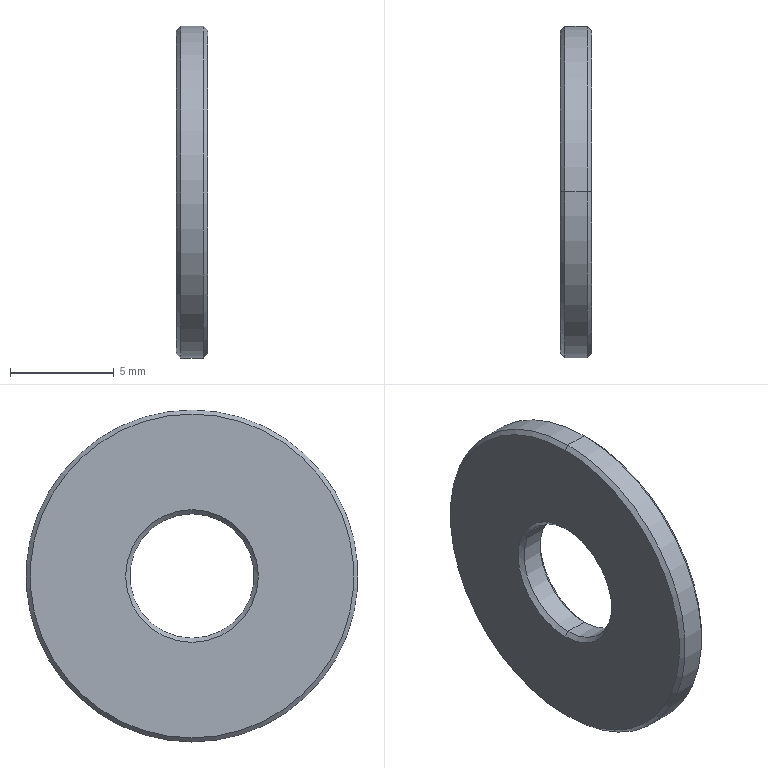Part | STEP file | WSSS16-6-1.5 | 1 solid | 14 faces | box 1.5 x 16 x 16 mm | volume 256.417 mm3 | cone 8 | cylinder 4 | plane 2 | commonest cylinder face diameters 6 x2 16 x2
STEP:
#1=CARTESIAN_POINT('',(0.,0.,0.));
#2=DIRECTION('',(0.,0.,1.));
#3=DIRECTION('',(1.,0.,0.));
#4=AXIS2_PLACEMENT_3D('',#1,#2,#3);
#5=CARTESIAN_POINT('',(1.5,0.,-7.8));
#6=VERTEX_POINT('',#5);
#7=CARTESIAN_POINT('',(1.5,0.,7.8));
#8=VERTEX_POINT('',#7);
#9=CARTESIAN_POINT('',(1.5,0.,0.));
#10=DIRECTION('',(1.,0.,0.));
#11=DIRECTION('',(0.,0.,1.));
#12=AXIS2_PLACEMENT_3D('',#9,#10,#11);
#13=CIRCLE('',#12,7.8);
#14=CARTESIAN_POINT('',(1.3,0.,0.));
#15=DIRECTION('',(-1.,0.,0.));
#16=DIRECTION('',(0.,0.,1.));
#17=AXIS2_PLACEMENT_3D('',#14,#15,#16);
#18=CONICAL_SURFACE('',#17,8.,0.7854);
#19=CARTESIAN_POINT('',(6.283,-0.2));
#20=DIRECTION('',(-1.,0.));
#21=VECTOR('',#20,1.);
#22=LINE('',#19,#21);
#23=(GEOMETRIC_REPRESENTATION_CONTEXT(2)PARAMETRIC_REPRESENTATION_CONTEXT()REPRESENTATION_CONTEXT('',''));
#24=DEFINITIONAL_REPRESENTATION('',(#22),#23);
#25=PCURVE('',#18,#24);
#26=CARTESIAN_POINT('',(1.5,3.,0.));
#27=DIRECTION('',(-1.,0.,0.));
#28=DIRECTION('',(0.,0.,1.));
#29=AXIS2_PLACEMENT_3D('',#26,#27,#28);
#30=PLANE('',#29);
#31=CARTESIAN_POINT('',(7.8,-3.));
#32=CARTESIAN_POINT('',(7.8,-16.51));
#33=CARTESIAN_POINT('',(-3.9,-9.755));
#34=CARTESIAN_POINT('',(-15.6,-3.));
#35=CARTESIAN_POINT('',(-3.9,3.755));
#36=CARTESIAN_POINT('',(7.8,10.51));
#37=CARTESIAN_POINT('',(7.8,-3.));
#38=(BOUNDED_CURVE()B_SPLINE_CURVE(2,(#31,#32,#33,#34,#35,#36,#37),.UNSPECIFIED.,.T.,.F.)B_SPLINE_CURVE_WITH_KNOTS((1,2,2,2,2,1),(-2.094,0.,2.094,4.189,6.283,8.378),.UNSPECIFIED.)CURVE()GEOMETRIC_REPRESENTATION_ITEM()RATIONAL_B_SPLINE_CURVE((1.,0.5,1.,0.5,1.,0.5,1.))REPRESENTATION_ITEM(''));
#39=(GEOMETRIC_REPRESENTATION_CONTEXT(2)PARAMETRIC_REPRESENTATION_CONTEXT()REPRESENTATION_CONTEXT('',''));
#40=DEFINITIONAL_REPRESENTATION('',(#38),#39);
#41=PCURVE('',#30,#40);
#42=SURFACE_CURVE('',#13,(#25,#41),.PCURVE_S1.);
#43=EDGE_CURVE('',#6,#8,#42,.T.);
#44=ORIENTED_EDGE('',*,*,#43,.F.);
#45=CARTESIAN_POINT('',(1.3,0.,-8.));
#46=VERTEX_POINT('',#45);
#47=CARTESIAN_POINT('',(1.3,0.,-8.));
#48=DIRECTION('',(-0.7071,0.,-0.7071));
#49=VECTOR('',#48,1.);
#50=LINE('',#47,#49);
#51=CARTESIAN_POINT('',(3.142,0.));
#52=DIRECTION('',(0.,1.));
#53=VECTOR('',#52,1.);
#54=LINE('',#51,#53);
#55=(GEOMETRIC_REPRESENTATION_CONTEXT(2)PARAMETRIC_REPRESENTATION_CONTEXT()REPRESENTATION_CONTEXT('',''));
#56=DEFINITIONAL_REPRESENTATION('',(#54),#55);
#57=PCURVE('',#18,#56);
#58=CARTESIAN_POINT('',(1.3,0.,0.));
#59=DIRECTION('',(-1.,0.,0.));
#60=DIRECTION('',(0.,0.,1.));
#61=AXIS2_PLACEMENT_3D('',#58,#59,#60);
#62=CONICAL_SURFACE('',#61,8.,0.7854);
#63=CARTESIAN_POINT('',(3.142,0.));
#64=DIRECTION('',(0.,1.));
#65=VECTOR('',#64,1.);
#66=LINE('',#63,#65);
#67=(GEOMETRIC_REPRESENTATION_CONTEXT(2)PARAMETRIC_REPRESENTATION_CONTEXT()REPRESENTATION_CONTEXT('',''));
#68=DEFINITIONAL_REPRESENTATION('',(#66),#67);
#69=PCURVE('',#62,#68);
#70=SURFACE_CURVE('',#50,(#57,#69),.PCURVE_S1.);
#71=EDGE_CURVE('',#6,#46,#70,.T.);
#72=ORIENTED_EDGE('',*,*,#71,.T.);
#73=CARTESIAN_POINT('',(1.3,0.,8.));
#74=VERTEX_POINT('',#73);
#75=CARTESIAN_POINT('',(1.3,0.,0.));
#76=DIRECTION('',(-1.,0.,0.));
#77=DIRECTION('',(0.,0.,1.));
#78=AXIS2_PLACEMENT_3D('',#75,#76,#77);
#79=CIRCLE('',#78,8.);
#80=CARTESIAN_POINT('',(0.,0.));
#81=DIRECTION('',(1.,0.));
#82=VECTOR('',#81,1.);
#83=LINE('',#80,#82);
#84=(GEOMETRIC_REPRESENTATION_CONTEXT(2)PARAMETRIC_REPRESENTATION_CONTEXT()REPRESENTATION_CONTEXT('',''));
#85=DEFINITIONAL_REPRESENTATION('',(#83),#84);
#86=PCURVE('',#18,#85);
#87=CARTESIAN_POINT('',(0.,0.,0.));
#88=DIRECTION('',(-1.,0.,0.));
#89=DIRECTION('',(0.,0.,1.));
#90=AXIS2_PLACEMENT_3D('',#87,#88,#89);
#91=CYLINDRICAL_SURFACE('',#90,8.);
#92=CARTESIAN_POINT('',(0.,-1.3));
#93=DIRECTION('',(1.,0.));
#94=VECTOR('',#93,1.);
#95=LINE('',#92,#94);
#96=(GEOMETRIC_REPRESENTATION_CONTEXT(2)PARAMETRIC_REPRESENTATION_CONTEXT()REPRESENTATION_CONTEXT('',''));
#97=DEFINITIONAL_REPRESENTATION('',(#95),#96);
#98=PCURVE('',#91,#97);
#99=SURFACE_CURVE('',#79,(#86,#98),.PCURVE_S1.);
#100=EDGE_CURVE('',#74,#46,#99,.T.);
#101=ORIENTED_EDGE('',*,*,#100,.F.);
#102=CARTESIAN_POINT('',(1.3,0.,8.));
#103=DIRECTION('',(-0.7071,0.,0.7071));
#104=VECTOR('',#103,1.);
#105=LINE('',#102,#104);
#106=CARTESIAN_POINT('',(0.,0.));
#107=DIRECTION('',(0.,1.));
#108=VECTOR('',#107,1.);
#109=LINE('',#106,#108);
#110=(GEOMETRIC_REPRESENTATION_CONTEXT(2)PARAMETRIC_REPRESENTATION_CONTEXT()REPRESENTATION_CONTEXT('',''));
#111=DEFINITIONAL_REPRESENTATION('',(#109),#110);
#112=PCURVE('',#18,#111);
#113=CARTESIAN_POINT('',(6.283,0.));
#114=DIRECTION('',(0.,1.));
#115=VECTOR('',#114,1.);
#116=LINE('',#113,#115);
#117=(GEOMETRIC_REPRESENTATION_CONTEXT(2)PARAMETRIC_REPRESENTATION_CONTEXT()REPRESENTATION_CONTEXT('',''));
#118=DEFINITIONAL_REPRESENTATION('',(#116),#117);
#119=PCURVE('',#62,#118);
#120=SURFACE_CURVE('',#105,(#112,#119),.PCURVE_S1.);
#121=EDGE_CURVE('',#8,#74,#120,.T.);
#122=ORIENTED_EDGE('',*,*,#121,.F.);
#123=EDGE_LOOP('',(#44,#72,#101,#122));
#124=FACE_BOUND('',#123,.T.);
#125=ADVANCED_FACE('',(#124),#18,.T.);
#126=CARTESIAN_POINT('',(1.3,0.,-3.));
#127=VERTEX_POINT('',#126);
#128=CARTESIAN_POINT('',(1.5,0.,-3.2));
#129=VERTEX_POINT('',#128);
#130=CARTESIAN_POINT('',(1.5,0.,-3.2));
#131=DIRECTION('',(0.7071,0.,-0.7071));
#132=VECTOR('',#131,1.);
#133=LINE('',#130,#132);
#134=CARTESIAN_POINT('',(1.5,0.,0.));
#135=DIRECTION('',(1.,0.,0.));
#136=DIRECTION('',(0.,0.,-1.));
#137=AXIS2_PLACEMENT_3D('',#134,#135,#136);
#138=CONICAL_SURFACE('',#137,3.2,0.7854);
#139=CARTESIAN_POINT('',(6.283,0.));
#140=DIRECTION('',(0.,1.));
#141=VECTOR('',#140,1.);
#142=LINE('',#139,#141);
#143=(GEOMETRIC_REPRESENTATION_CONTEXT(2)PARAMETRIC_REPRESENTATION_CONTEXT()REPRESENTATION_CONTEXT('',''));
#144=DEFINITIONAL_REPRESENTATION('',(#142),#143);
#145=PCURVE('',#138,#144);
#146=CARTESIAN_POINT('',(1.5,0.,0.));
#147=DIRECTION('',(1.,0.,0.));
#148=DIRECTION('',(0.,0.,-1.));
#149=AXIS2_PLACEMENT_3D('',#146,#147,#148);
#150=CONICAL_SURFACE('',#149,3.2,0.7854);
#151=CARTESIAN_POINT('',(0.,0.));
#152=DIRECTION('',(0.,1.));
#153=VECTOR('',#152,1.);
#154=LINE('',#151,#153);
#155=(GEOMETRIC_REPRESENTATION_CONTEXT(2)PARAMETRIC_REPRESENTATION_CONTEXT()REPRESENTATION_CONTEXT('',''));
#156=DEFINITIONAL_REPRESENTATION('',(#154),#155);
#157=PCURVE('',#150,#156);
#158=SURFACE_CURVE('',#133,(#145,#157),.PCURVE_S1.);
#159=EDGE_CURVE('',#127,#129,#158,.T.);
#160=ORIENTED_EDGE('',*,*,#159,.T.);
#161=CARTESIAN_POINT('',(1.5,0.,3.2));
#162=VERTEX_POINT('',#161);
#163=CARTESIAN_POINT('',(1.5,0.,0.));
#164=DIRECTION('',(-1.,0.,0.));
#165=DIRECTION('',(0.,0.,1.));
#166=AXIS2_PLACEMENT_3D('',#163,#164,#165);
#167=CIRCLE('',#166,3.2);
#168=CARTESIAN_POINT('',(9.425,0.));
#169=DIRECTION('',(-1.,0.));
#170=VECTOR('',#169,1.);
#171=LINE('',#168,#170);
#172=(GEOMETRIC_REPRESENTATION_CONTEXT(2)PARAMETRIC_REPRESENTATION_CONTEXT()REPRESENTATION_CONTEXT('',''));
#173=DEFINITIONAL_REPRESENTATION('',(#171),#172);
#174=PCURVE('',#138,#173);
#175=CARTESIAN_POINT('',(0.,-3.));
#176=DIRECTION('',(1.,0.));
#177=AXIS2_PLACEMENT_2D('',#175,#176);
#178=CIRCLE('',#177,3.2);
#179=(GEOMETRIC_REPRESENTATION_CONTEXT(2)PARAMETRIC_REPRESENTATION_CONTEXT()REPRESENTATION_CONTEXT('',''));
#180=DEFINITIONAL_REPRESENTATION('',(#178),#179);
#181=PCURVE('',#30,#180);
#182=SURFACE_CURVE('',#167,(#174,#181),.PCURVE_S1.);
#183=EDGE_CURVE('',#129,#162,#182,.T.);
#184=ORIENTED_EDGE('',*,*,#183,.T.);
#185=CARTESIAN_POINT('',(1.3,0.,3.));
#186=VERTEX_POINT('',#185);
#187=CARTESIAN_POINT('',(1.5,0.,3.2));
#188=DIRECTION('',(0.7071,0.,0.7071));
#189=VECTOR('',#188,1.);
#190=LINE('',#187,#189);
#191=CARTESIAN_POINT('',(3.142,0.));
#192=DIRECTION('',(0.,1.));
#193=VECTOR('',#192,1.);
#194=LINE('',#191,#193);
#195=(GEOMETRIC_REPRESENTATION_CONTEXT(2)PARAMETRIC_REPRESENTATION_CONTEXT()REPRESENTATION_CONTEXT('',''));
#196=DEFINITIONAL_REPRESENTATION('',(#194),#195);
#197=PCURVE('',#138,#196);
#198=CARTESIAN_POINT('',(3.142,0.));
#199=DIRECTION('',(0.,1.));
#200=VECTOR('',#199,1.);
#201=LINE('',#198,#200);
#202=(GEOMETRIC_REPRESENTATION_CONTEXT(2)PARAMETRIC_REPRESENTATION_CONTEXT()REPRESENTATION_CONTEXT('',''));
#203=DEFINITIONAL_REPRESENTATION('',(#201),#202);
#204=PCURVE('',#150,#203);
#205=SURFACE_CURVE('',#190,(#197,#204),.PCURVE_S1.);
#206=EDGE_CURVE('',#186,#162,#205,.T.);
#207=ORIENTED_EDGE('',*,*,#206,.F.);
#208=CARTESIAN_POINT('',(1.3,0.,0.));
#209=DIRECTION('',(1.,0.,0.));
#210=DIRECTION('',(0.,0.,1.));
#211=AXIS2_PLACEMENT_3D('',#208,#209,#210);
#212=CIRCLE('',#211,3.);
#213=CARTESIAN_POINT('',(3.142,-0.2));
#214=DIRECTION('',(1.,0.));
#215=VECTOR('',#214,1.);
#216=LINE('',#213,#215);
#217=(GEOMETRIC_REPRESENTATION_CONTEXT(2)PARAMETRIC_REPRESENTATION_CONTEXT()REPRESENTATION_CONTEXT('',''));
#218=DEFINITIONAL_REPRESENTATION('',(#216),#217);
#219=PCURVE('',#138,#218);
#220=CARTESIAN_POINT('',(0.,0.,0.));
#221=DIRECTION('',(-1.,0.,0.));
#222=DIRECTION('',(0.,0.,1.));
#223=AXIS2_PLACEMENT_3D('',#220,#221,#222);
#224=CYLINDRICAL_SURFACE('',#223,3.);
#225=CARTESIAN_POINT('',(6.283,-1.3));
#226=DIRECTION('',(-1.,0.));
#227=VECTOR('',#226,1.);
#228=LINE('',#225,#227);
#229=(GEOMETRIC_REPRESENTATION_CONTEXT(2)PARAMETRIC_REPRESENTATION_CONTEXT()REPRESENTATION_CONTEXT('',''));
#230=DEFINITIONAL_REPRESENTATION('',(#228),#229);
#231=PCURVE('',#224,#230);
#232=SURFACE_CURVE('',#212,(#219,#231),.PCURVE_S1.);
#233=EDGE_CURVE('',#186,#127,#232,.T.);
#234=ORIENTED_EDGE('',*,*,#233,.T.);
#235=EDGE_LOOP('',(#160,#184,#207,#234));
#236=FACE_BOUND('',#235,.F.);
#237=ADVANCED_FACE('',(#236),#138,.F.);
#238=CARTESIAN_POINT('',(0.,0.,7.8));
#239=VERTEX_POINT('',#238);
#240=CARTESIAN_POINT('',(0.,0.,-7.8));
#241=VERTEX_POINT('',#240);
#242=CARTESIAN_POINT('',(0.,0.,0.));
#243=DIRECTION('',(-1.,0.,0.));
#244=DIRECTION('',(0.,0.,-1.));
#245=AXIS2_PLACEMENT_3D('',#242,#243,#244);
#246=CIRCLE('',#245,7.8);
#247=CARTESIAN_POINT('',(0.,0.,0.));
#248=DIRECTION('',(1.,0.,0.));
#249=DIRECTION('',(0.,0.,-1.));
#250=AXIS2_PLACEMENT_3D('',#247,#248,#249);
#251=CONICAL_SURFACE('',#250,7.8,0.7854);
#252=CARTESIAN_POINT('',(6.283,0.));
#253=DIRECTION('',(-1.,0.));
#254=VECTOR('',#253,1.);
#255=LINE('',#252,#254);
#256=(GEOMETRIC_REPRESENTATION_CONTEXT(2)PARAMETRIC_REPRESENTATION_CONTEXT()REPRESENTATION_CONTEXT('',''));
#257=DEFINITIONAL_REPRESENTATION('',(#255),#256);
#258=PCURVE('',#251,#257);
#259=CARTESIAN_POINT('',(0.,3.,0.));
#260=DIRECTION('',(1.,0.,0.));
#261=DIRECTION('',(0.,0.,-1.));
#262=AXIS2_PLACEMENT_3D('',#259,#260,#261);
#263=PLANE('',#262);
#264=CARTESIAN_POINT('',(7.8,-3.));
#265=CARTESIAN_POINT('',(7.8,-16.51));
#266=CARTESIAN_POINT('',(-3.9,-9.755));
#267=CARTESIAN_POINT('',(-15.6,-3.));
#268=CARTESIAN_POINT('',(-3.9,3.755));
#269=CARTESIAN_POINT('',(7.8,10.51));
#270=CARTESIAN_POINT('',(7.8,-3.));
#271=(BOUNDED_CURVE()B_SPLINE_CURVE(2,(#264,#265,#266,#267,#268,#269,#270),.UNSPECIFIED.,.T.,.F.)B_SPLINE_CURVE_WITH_KNOTS((1,2,2,2,2,1),(-2.094,0.,2.094,4.189,6.283,8.378),.UNSPECIFIED.)CURVE()GEOMETRIC_REPRESENTATION_ITEM()RATIONAL_B_SPLINE_CURVE((1.,0.5,1.,0.5,1.,0.5,1.))REPRESENTATION_ITEM(''));
#272=(GEOMETRIC_REPRESENTATION_CONTEXT(2)PARAMETRIC_REPRESENTATION_CONTEXT()REPRESENTATION_CONTEXT('',''));
#273=DEFINITIONAL_REPRESENTATION('',(#271),#272);
#274=PCURVE('',#263,#273);
#275=SURFACE_CURVE('',#246,(#258,#274),.PCURVE_S1.);
#276=EDGE_CURVE('',#239,#241,#275,.T.);
#277=ORIENTED_EDGE('',*,*,#276,.F.);
#278=CARTESIAN_POINT('',(0.2,0.,8.));
#279=VERTEX_POINT('',#278);
#280=CARTESIAN_POINT('',(0.,0.,7.8));
#281=DIRECTION('',(0.7071,0.,0.7071));
#282=VECTOR('',#281,1.);
#283=LINE('',#280,#282);
#284=CARTESIAN_POINT('',(3.142,0.));
#285=DIRECTION('',(0.,1.));
#286=VECTOR('',#285,1.);
#287=LINE('',#284,#286);
#288=(GEOMETRIC_REPRESENTATION_CONTEXT(2)PARAMETRIC_REPRESENTATION_CONTEXT()REPRESENTATION_CONTEXT('',''));
#289=DEFINITIONAL_REPRESENTATION('',(#287),#288);
#290=PCURVE('',#251,#289);
#291=CARTESIAN_POINT('',(0.,0.,0.));
#292=DIRECTION('',(1.,0.,0.));
#293=DIRECTION('',(0.,0.,-1.));
#294=AXIS2_PLACEMENT_3D('',#291,#292,#293);
#295=CONICAL_SURFACE('',#294,7.8,0.7854);
#296=CARTESIAN_POINT('',(3.142,0.));
#297=DIRECTION('',(0.,1.));
#298=VECTOR('',#297,1.);
#299=LINE('',#296,#298);
#300=(GEOMETRIC_REPRESENTATION_CONTEXT(2)PARAMETRIC_REPRESENTATION_CONTEXT()REPRESENTATION_CONTEXT('',''));
#301=DEFINITIONAL_REPRESENTATION('',(#299),#300);
#302=PCURVE('',#295,#301);
#303=SURFACE_CURVE('',#283,(#290,#302),.PCURVE_S1.);
#304=EDGE_CURVE('',#239,#279,#303,.T.);
#305=ORIENTED_EDGE('',*,*,#304,.T.);
#306=CARTESIAN_POINT('',(0.2,0.,-8.));
#307=VERTEX_POINT('',#306);
#308=CARTESIAN_POINT('',(0.2,0.,0.));
#309=DIRECTION('',(1.,0.,0.));
#310=DIRECTION('',(0.,0.,-1.));
#311=AXIS2_PLACEMENT_3D('',#308,#309,#310);
#312=CIRCLE('',#311,8.);
#313=CARTESIAN_POINT('',(0.,0.2));
#314=DIRECTION('',(1.,0.));
#315=VECTOR('',#314,1.);
#316=LINE('',#313,#315);
#317=(GEOMETRIC_REPRESENTATION_CONTEXT(2)PARAMETRIC_REPRESENTATION_CONTEXT()REPRESENTATION_CONTEXT('',''));
#318=DEFINITIONAL_REPRESENTATION('',(#316),#317);
#319=PCURVE('',#251,#318);
#320=CARTESIAN_POINT('',(3.142,-0.2));
#321=DIRECTION('',(-1.,0.));
#322=VECTOR('',#321,1.);
#323=LINE('',#320,#322);
#324=(GEOMETRIC_REPRESENTATION_CONTEXT(2)PARAMETRIC_REPRESENTATION_CONTEXT()REPRESENTATION_CONTEXT('',''));
#325=DEFINITIONAL_REPRESENTATION('',(#323),#324);
#326=PCURVE('',#91,#325);
#327=SURFACE_CURVE('',#312,(#319,#326),.PCURVE_S1.);
#328=EDGE_CURVE('',#307,#279,#327,.T.);
#329=ORIENTED_EDGE('',*,*,#328,.F.);
#330=CARTESIAN_POINT('',(0.,0.,-7.8));
#331=DIRECTION('',(0.7071,0.,-0.7071));
#332=VECTOR('',#331,1.);
#333=LINE('',#330,#332);
#334=CARTESIAN_POINT('',(0.,0.));
#335=DIRECTION('',(0.,1.));
#336=VECTOR('',#335,1.);
#337=LINE('',#334,#336);
#338=(GEOMETRIC_REPRESENTATION_CONTEXT(2)PARAMETRIC_REPRESENTATION_CONTEXT()REPRESENTATION_CONTEXT('',''));
#339=DEFINITIONAL_REPRESENTATION('',(#337),#338);
#340=PCURVE('',#251,#339);
#341=CARTESIAN_POINT('',(6.283,0.));
#342=DIRECTION('',(0.,1.));
#343=VECTOR('',#342,1.);
#344=LINE('',#341,#343);
#345=(GEOMETRIC_REPRESENTATION_CONTEXT(2)PARAMETRIC_REPRESENTATION_CONTEXT()REPRESENTATION_CONTEXT('',''));
#346=DEFINITIONAL_REPRESENTATION('',(#344),#345);
#347=PCURVE('',#295,#346);
#348=SURFACE_CURVE('',#333,(#340,#347),.PCURVE_S1.);
#349=EDGE_CURVE('',#241,#307,#348,.T.);
#350=ORIENTED_EDGE('',*,*,#349,.F.);
#351=EDGE_LOOP('',(#277,#305,#329,#350));
#352=FACE_BOUND('',#351,.T.);
#353=ADVANCED_FACE('',(#352),#251,.T.);
#354=CARTESIAN_POINT('',(0.2,0.,3.));
#355=VERTEX_POINT('',#354);
#356=CARTESIAN_POINT('',(0.,0.,3.2));
#357=VERTEX_POINT('',#356);
#358=CARTESIAN_POINT('',(0.2,0.,3.));
#359=DIRECTION('',(-0.7071,0.,0.7071));
#360=VECTOR('',#359,1.);
#361=LINE('',#358,#360);
#362=CARTESIAN_POINT('',(0.2,0.,0.));
#363=DIRECTION('',(-1.,0.,0.));
#364=DIRECTION('',(0.,0.,1.));
#365=AXIS2_PLACEMENT_3D('',#362,#363,#364);
#366=CONICAL_SURFACE('',#365,3.,0.7854);
#367=CARTESIAN_POINT('',(6.283,0.));
#368=DIRECTION('',(0.,1.));
#369=VECTOR('',#368,1.);
#370=LINE('',#367,#369);
#371=(GEOMETRIC_REPRESENTATION_CONTEXT(2)PARAMETRIC_REPRESENTATION_CONTEXT()REPRESENTATION_CONTEXT('',''));
#372=DEFINITIONAL_REPRESENTATION('',(#370),#371);
#373=PCURVE('',#366,#372);
#374=CARTESIAN_POINT('',(0.2,0.,0.));
#375=DIRECTION('',(-1.,0.,0.));
#376=DIRECTION('',(0.,0.,1.));
#377=AXIS2_PLACEMENT_3D('',#374,#375,#376);
#378=CONICAL_SURFACE('',#377,3.,0.7854);
#379=CARTESIAN_POINT('',(0.,0.));
#380=DIRECTION('',(0.,1.));
#381=VECTOR('',#380,1.);
#382=LINE('',#379,#381);
#383=(GEOMETRIC_REPRESENTATION_CONTEXT(2)PARAMETRIC_REPRESENTATION_CONTEXT()REPRESENTATION_CONTEXT('',''));
#384=DEFINITIONAL_REPRESENTATION('',(#382),#383);
#385=PCURVE('',#378,#384);
#386=SURFACE_CURVE('',#361,(#373,#385),.PCURVE_S1.);
#387=EDGE_CURVE('',#355,#357,#386,.T.);
#388=ORIENTED_EDGE('',*,*,#387,.T.);
#389=CARTESIAN_POINT('',(0.,0.,-3.2));
#390=VERTEX_POINT('',#389);
#391=CARTESIAN_POINT('',(0.,0.,0.));
#392=DIRECTION('',(1.,0.,0.));
#393=DIRECTION('',(0.,0.,-1.));
#394=AXIS2_PLACEMENT_3D('',#391,#392,#393);
#395=CIRCLE('',#394,3.2);
#396=CARTESIAN_POINT('',(9.425,0.2));
#397=DIRECTION('',(-1.,0.));
#398=VECTOR('',#397,1.);
#399=LINE('',#396,#398);
#400=(GEOMETRIC_REPRESENTATION_CONTEXT(2)PARAMETRIC_REPRESENTATION_CONTEXT()REPRESENTATION_CONTEXT('',''));
#401=DEFINITIONAL_REPRESENTATION('',(#399),#400);
#402=PCURVE('',#366,#401);
#403=CARTESIAN_POINT('',(0.,-3.));
#404=DIRECTION('',(1.,0.));
#405=AXIS2_PLACEMENT_2D('',#403,#404);
#406=CIRCLE('',#405,3.2);
#407=(GEOMETRIC_REPRESENTATION_CONTEXT(2)PARAMETRIC_REPRESENTATION_CONTEXT()REPRESENTATION_CONTEXT('',''));
#408=DEFINITIONAL_REPRESENTATION('',(#406),#407);
#409=PCURVE('',#263,#408);
#410=SURFACE_CURVE('',#395,(#402,#409),.PCURVE_S1.);
#411=EDGE_CURVE('',#357,#390,#410,.T.);
#412=ORIENTED_EDGE('',*,*,#411,.T.);
#413=CARTESIAN_POINT('',(0.2,0.,-3.));
#414=VERTEX_POINT('',#413);
#415=CARTESIAN_POINT('',(0.2,0.,-3.));
#416=DIRECTION('',(-0.7071,0.,-0.7071));
#417=VECTOR('',#416,1.);
#418=LINE('',#415,#417);
#419=CARTESIAN_POINT('',(3.142,0.));
#420=DIRECTION('',(0.,1.));
#421=VECTOR('',#420,1.);
#422=LINE('',#419,#421);
#423=(GEOMETRIC_REPRESENTATION_CONTEXT(2)PARAMETRIC_REPRESENTATION_CONTEXT()REPRESENTATION_CONTEXT('',''));
#424=DEFINITIONAL_REPRESENTATION('',(#422),#423);
#425=PCURVE('',#366,#424);
#426=CARTESIAN_POINT('',(3.142,0.));
#427=DIRECTION('',(0.,1.));
#428=VECTOR('',#427,1.);
#429=LINE('',#426,#428);
#430=(GEOMETRIC_REPRESENTATION_CONTEXT(2)PARAMETRIC_REPRESENTATION_CONTEXT()REPRESENTATION_CONTEXT('',''));
#431=DEFINITIONAL_REPRESENTATION('',(#429),#430);
#432=PCURVE('',#378,#431);
#433=SURFACE_CURVE('',#418,(#425,#432),.PCURVE_S1.);
#434=EDGE_CURVE('',#414,#390,#433,.T.);
#435=ORIENTED_EDGE('',*,*,#434,.F.);
#436=CARTESIAN_POINT('',(0.2,0.,0.));
#437=DIRECTION('',(-1.,0.,0.));
#438=DIRECTION('',(0.,0.,-1.));
#439=AXIS2_PLACEMENT_3D('',#436,#437,#438);
#440=CIRCLE('',#439,3.);
#441=CARTESIAN_POINT('',(3.142,0.));
#442=DIRECTION('',(1.,0.));
#443=VECTOR('',#442,1.);
#444=LINE('',#441,#443);
#445=(GEOMETRIC_REPRESENTATION_CONTEXT(2)PARAMETRIC_REPRESENTATION_CONTEXT()REPRESENTATION_CONTEXT('',''));
#446=DEFINITIONAL_REPRESENTATION('',(#444),#445);
#447=PCURVE('',#366,#446);
#448=CARTESIAN_POINT('',(3.142,-0.2));
#449=DIRECTION('',(1.,0.));
#450=VECTOR('',#449,1.);
#451=LINE('',#448,#450);
#452=(GEOMETRIC_REPRESENTATION_CONTEXT(2)PARAMETRIC_REPRESENTATION_CONTEXT()REPRESENTATION_CONTEXT('',''));
#453=DEFINITIONAL_REPRESENTATION('',(#451),#452);
#454=PCURVE('',#224,#453);
#455=SURFACE_CURVE('',#440,(#447,#454),.PCURVE_S1.);
#456=EDGE_CURVE('',#414,#355,#455,.T.);
#457=ORIENTED_EDGE('',*,*,#456,.T.);
#458=EDGE_LOOP('',(#388,#412,#435,#457));
#459=FACE_BOUND('',#458,.F.);
#460=ADVANCED_FACE('',(#459),#366,.F.);
#461=CARTESIAN_POINT('',(0.,0.,3.));
#462=DIRECTION('',(-1.,0.,0.));
#463=VECTOR('',#462,1.);
#464=LINE('',#461,#463);
#465=CARTESIAN_POINT('',(6.283,0.));
#466=DIRECTION('',(0.,1.));
#467=VECTOR('',#466,1.);
#468=LINE('',#465,#467);
#469=(GEOMETRIC_REPRESENTATION_CONTEXT(2)PARAMETRIC_REPRESENTATION_CONTEXT()REPRESENTATION_CONTEXT('',''));
#470=DEFINITIONAL_REPRESENTATION('',(#468),#469);
#471=PCURVE('',#224,#470);
#472=CARTESIAN_POINT('',(0.,0.,0.));
#473=DIRECTION('',(-1.,0.,0.));
#474=DIRECTION('',(0.,0.,1.));
#475=AXIS2_PLACEMENT_3D('',#472,#473,#474);
#476=CYLINDRICAL_SURFACE('',#475,3.);
#477=CARTESIAN_POINT('',(0.,0.));
#478=DIRECTION('',(0.,1.));
#479=VECTOR('',#478,1.);
#480=LINE('',#477,#479);
#481=(GEOMETRIC_REPRESENTATION_CONTEXT(2)PARAMETRIC_REPRESENTATION_CONTEXT()REPRESENTATION_CONTEXT('',''));
#482=DEFINITIONAL_REPRESENTATION('',(#480),#481);
#483=PCURVE('',#476,#482);
#484=SURFACE_CURVE('',#464,(#471,#483),.PCURVE_S1.);
#485=EDGE_CURVE('',#186,#355,#484,.T.);
#486=ORIENTED_EDGE('',*,*,#485,.T.);
#487=ORIENTED_EDGE('',*,*,#456,.F.);
#488=CARTESIAN_POINT('',(0.,0.,-3.));
#489=DIRECTION('',(-1.,0.,0.));
#490=VECTOR('',#489,1.);
#491=LINE('',#488,#490);
#492=CARTESIAN_POINT('',(3.142,0.));
#493=DIRECTION('',(0.,1.));
#494=VECTOR('',#493,1.);
#495=LINE('',#492,#494);
#496=(GEOMETRIC_REPRESENTATION_CONTEXT(2)PARAMETRIC_REPRESENTATION_CONTEXT()REPRESENTATION_CONTEXT('',''));
#497=DEFINITIONAL_REPRESENTATION('',(#495),#496);
#498=PCURVE('',#224,#497);
#499=CARTESIAN_POINT('',(3.142,0.));
#500=DIRECTION('',(0.,1.));
#501=VECTOR('',#500,1.);
#502=LINE('',#499,#501);
#503=(GEOMETRIC_REPRESENTATION_CONTEXT(2)PARAMETRIC_REPRESENTATION_CONTEXT()REPRESENTATION_CONTEXT('',''));
#504=DEFINITIONAL_REPRESENTATION('',(#502),#503);
#505=PCURVE('',#476,#504);
#506=SURFACE_CURVE('',#491,(#498,#505),.PCURVE_S1.);
#507=EDGE_CURVE('',#127,#414,#506,.T.);
#508=ORIENTED_EDGE('',*,*,#507,.F.);
#509=ORIENTED_EDGE('',*,*,#233,.F.);
#510=EDGE_LOOP('',(#486,#487,#508,#509));
#511=FACE_BOUND('',#510,.F.);
#512=ADVANCED_FACE('',(#511),#224,.F.);
#513=ORIENTED_EDGE('',*,*,#100,.T.);
#514=CARTESIAN_POINT('',(0.,0.,-8.));
#515=DIRECTION('',(-1.,0.,0.));
#516=VECTOR('',#515,1.);
#517=LINE('',#514,#516);
#518=CARTESIAN_POINT('',(3.142,0.));
#519=DIRECTION('',(0.,1.));
#520=VECTOR('',#519,1.);
#521=LINE('',#518,#520);
#522=(GEOMETRIC_REPRESENTATION_CONTEXT(2)PARAMETRIC_REPRESENTATION_CONTEXT()REPRESENTATION_CONTEXT('',''));
#523=DEFINITIONAL_REPRESENTATION('',(#521),#522);
#524=PCURVE('',#91,#523);
#525=CARTESIAN_POINT('',(0.,0.,0.));
#526=DIRECTION('',(-1.,0.,0.));
#527=DIRECTION('',(0.,0.,1.));
#528=AXIS2_PLACEMENT_3D('',#525,#526,#527);
#529=CYLINDRICAL_SURFACE('',#528,8.);
#530=CARTESIAN_POINT('',(3.142,0.));
#531=DIRECTION('',(0.,1.));
#532=VECTOR('',#531,1.);
#533=LINE('',#530,#532);
#534=(GEOMETRIC_REPRESENTATION_CONTEXT(2)PARAMETRIC_REPRESENTATION_CONTEXT()REPRESENTATION_CONTEXT('',''));
#535=DEFINITIONAL_REPRESENTATION('',(#533),#534);
#536=PCURVE('',#529,#535);
#537=SURFACE_CURVE('',#517,(#524,#536),.PCURVE_S1.);
#538=EDGE_CURVE('',#46,#307,#537,.T.);
#539=ORIENTED_EDGE('',*,*,#538,.T.);
#540=ORIENTED_EDGE('',*,*,#328,.T.);
#541=CARTESIAN_POINT('',(0.,0.,8.));
#542=DIRECTION('',(-1.,0.,0.));
#543=VECTOR('',#542,1.);
#544=LINE('',#541,#543);
#545=CARTESIAN_POINT('',(0.,0.));
#546=DIRECTION('',(0.,1.));
#547=VECTOR('',#546,1.);
#548=LINE('',#545,#547);
#549=(GEOMETRIC_REPRESENTATION_CONTEXT(2)PARAMETRIC_REPRESENTATION_CONTEXT()REPRESENTATION_CONTEXT('',''));
#550=DEFINITIONAL_REPRESENTATION('',(#548),#549);
#551=PCURVE('',#91,#550);
#552=CARTESIAN_POINT('',(6.283,0.));
#553=DIRECTION('',(0.,1.));
#554=VECTOR('',#553,1.);
#555=LINE('',#552,#554);
#556=(GEOMETRIC_REPRESENTATION_CONTEXT(2)PARAMETRIC_REPRESENTATION_CONTEXT()REPRESENTATION_CONTEXT('',''));
#557=DEFINITIONAL_REPRESENTATION('',(#555),#556);
#558=PCURVE('',#529,#557);
#559=SURFACE_CURVE('',#544,(#551,#558),.PCURVE_S1.);
#560=EDGE_CURVE('',#74,#279,#559,.T.);
#561=ORIENTED_EDGE('',*,*,#560,.F.);
#562=EDGE_LOOP('',(#513,#539,#540,#561));
#563=FACE_BOUND('',#562,.T.);
#564=ADVANCED_FACE('',(#563),#91,.T.);
#565=ORIENTED_EDGE('',*,*,#411,.T.);
#566=CARTESIAN_POINT('',(0.,0.,0.));
#567=DIRECTION('',(1.,0.,0.));
#568=DIRECTION('',(0.,0.,-1.));
#569=AXIS2_PLACEMENT_3D('',#566,#567,#568);
#570=CIRCLE('',#569,3.2);
#571=CARTESIAN_POINT('',(0.,-3.));
#572=DIRECTION('',(1.,0.));
#573=AXIS2_PLACEMENT_2D('',#571,#572);
#574=CIRCLE('',#573,3.2);
#575=(GEOMETRIC_REPRESENTATION_CONTEXT(2)PARAMETRIC_REPRESENTATION_CONTEXT()REPRESENTATION_CONTEXT('',''));
#576=DEFINITIONAL_REPRESENTATION('',(#574),#575);
#577=PCURVE('',#263,#576);
#578=CARTESIAN_POINT('',(3.142,0.2));
#579=DIRECTION('',(-1.,0.));
#580=VECTOR('',#579,1.);
#581=LINE('',#578,#580);
#582=(GEOMETRIC_REPRESENTATION_CONTEXT(2)PARAMETRIC_REPRESENTATION_CONTEXT()REPRESENTATION_CONTEXT('',''));
#583=DEFINITIONAL_REPRESENTATION('',(#581),#582);
#584=PCURVE('',#378,#583);
#585=SURFACE_CURVE('',#570,(#577,#584),.PCURVE_S1.);
#586=EDGE_CURVE('',#390,#357,#585,.T.);
#587=ORIENTED_EDGE('',*,*,#586,.T.);
#588=EDGE_LOOP('',(#565,#587));
#589=FACE_BOUND('',#588,.T.);
#590=CARTESIAN_POINT('',(0.,0.,0.));
#591=DIRECTION('',(-1.,0.,0.));
#592=DIRECTION('',(0.,0.,-1.));
#593=AXIS2_PLACEMENT_3D('',#590,#591,#592);
#594=CIRCLE('',#593,7.8);
#595=CARTESIAN_POINT('',(7.8,-3.));
#596=CARTESIAN_POINT('',(7.8,-16.51));
#597=CARTESIAN_POINT('',(-3.9,-9.755));
#598=CARTESIAN_POINT('',(-15.6,-3.));
#599=CARTESIAN_POINT('',(-3.9,3.755));
#600=CARTESIAN_POINT('',(7.8,10.51));
#601=CARTESIAN_POINT('',(7.8,-3.));
#602=(BOUNDED_CURVE()B_SPLINE_CURVE(2,(#595,#596,#597,#598,#599,#600,#601),.UNSPECIFIED.,.T.,.F.)B_SPLINE_CURVE_WITH_KNOTS((1,2,2,2,2,1),(-2.094,0.,2.094,4.189,6.283,8.378),.UNSPECIFIED.)CURVE()GEOMETRIC_REPRESENTATION_ITEM()RATIONAL_B_SPLINE_CURVE((1.,0.5,1.,0.5,1.,0.5,1.))REPRESENTATION_ITEM(''));
#603=(GEOMETRIC_REPRESENTATION_CONTEXT(2)PARAMETRIC_REPRESENTATION_CONTEXT()REPRESENTATION_CONTEXT('',''));
#604=DEFINITIONAL_REPRESENTATION('',(#602),#603);
#605=PCURVE('',#263,#604);
#606=CARTESIAN_POINT('',(6.283,0.));
#607=DIRECTION('',(-1.,0.));
#608=VECTOR('',#607,1.);
#609=LINE('',#606,#608);
#610=(GEOMETRIC_REPRESENTATION_CONTEXT(2)PARAMETRIC_REPRESENTATION_CONTEXT()REPRESENTATION_CONTEXT('',''));
#611=DEFINITIONAL_REPRESENTATION('',(#609),#610);
#612=PCURVE('',#295,#611);
#613=SURFACE_CURVE('',#594,(#605,#612),.PCURVE_S1.);
#614=EDGE_CURVE('',#241,#239,#613,.T.);
#615=ORIENTED_EDGE('',*,*,#614,.T.);
#616=ORIENTED_EDGE('',*,*,#276,.T.);
#617=EDGE_LOOP('',(#615,#616));
#618=FACE_BOUND('',#617,.T.);
#619=ADVANCED_FACE('',(#589,#618),#263,.F.);
#620=ORIENTED_EDGE('',*,*,#538,.F.);
#621=CARTESIAN_POINT('',(1.3,0.,0.));
#622=DIRECTION('',(-1.,0.,0.));
#623=DIRECTION('',(0.,0.,1.));
#624=AXIS2_PLACEMENT_3D('',#621,#622,#623);
#625=CIRCLE('',#624,8.);
#626=CARTESIAN_POINT('',(0.,-1.3));
#627=DIRECTION('',(1.,0.));
#628=VECTOR('',#627,1.);
#629=LINE('',#626,#628);
#630=(GEOMETRIC_REPRESENTATION_CONTEXT(2)PARAMETRIC_REPRESENTATION_CONTEXT()REPRESENTATION_CONTEXT('',''));
#631=DEFINITIONAL_REPRESENTATION('',(#629),#630);
#632=PCURVE('',#529,#631);
#633=CARTESIAN_POINT('',(0.,0.));
#634=DIRECTION('',(1.,0.));
#635=VECTOR('',#634,1.);
#636=LINE('',#633,#635);
#637=(GEOMETRIC_REPRESENTATION_CONTEXT(2)PARAMETRIC_REPRESENTATION_CONTEXT()REPRESENTATION_CONTEXT('',''));
#638=DEFINITIONAL_REPRESENTATION('',(#636),#637);
#639=PCURVE('',#62,#638);
#640=SURFACE_CURVE('',#625,(#632,#639),.PCURVE_S1.);
#641=EDGE_CURVE('',#46,#74,#640,.T.);
#642=ORIENTED_EDGE('',*,*,#641,.T.);
#643=ORIENTED_EDGE('',*,*,#560,.T.);
#644=CARTESIAN_POINT('',(0.2,0.,0.));
#645=DIRECTION('',(1.,0.,0.));
#646=DIRECTION('',(0.,0.,-1.));
#647=AXIS2_PLACEMENT_3D('',#644,#645,#646);
#648=CIRCLE('',#647,8.);
#649=CARTESIAN_POINT('',(9.425,-0.2));
#650=DIRECTION('',(-1.,0.));
#651=VECTOR('',#650,1.);
#652=LINE('',#649,#651);
#653=(GEOMETRIC_REPRESENTATION_CONTEXT(2)PARAMETRIC_REPRESENTATION_CONTEXT()REPRESENTATION_CONTEXT('',''));
#654=DEFINITIONAL_REPRESENTATION('',(#652),#653);
#655=PCURVE('',#529,#654);
#656=CARTESIAN_POINT('',(0.,0.2));
#657=DIRECTION('',(1.,0.));
#658=VECTOR('',#657,1.);
#659=LINE('',#656,#658);
#660=(GEOMETRIC_REPRESENTATION_CONTEXT(2)PARAMETRIC_REPRESENTATION_CONTEXT()REPRESENTATION_CONTEXT('',''));
#661=DEFINITIONAL_REPRESENTATION('',(#659),#660);
#662=PCURVE('',#295,#661);
#663=SURFACE_CURVE('',#648,(#655,#662),.PCURVE_S1.);
#664=EDGE_CURVE('',#279,#307,#663,.T.);
#665=ORIENTED_EDGE('',*,*,#664,.T.);
#666=EDGE_LOOP('',(#620,#642,#643,#665));
#667=FACE_BOUND('',#666,.T.);
#668=ADVANCED_FACE('',(#667),#529,.T.);
#669=ORIENTED_EDGE('',*,*,#183,.T.);
#670=CARTESIAN_POINT('',(1.5,0.,0.));
#671=DIRECTION('',(-1.,0.,0.));
#672=DIRECTION('',(0.,0.,1.));
#673=AXIS2_PLACEMENT_3D('',#670,#671,#672);
#674=CIRCLE('',#673,3.2);
#675=CARTESIAN_POINT('',(0.,-3.));
#676=DIRECTION('',(1.,0.));
#677=AXIS2_PLACEMENT_2D('',#675,#676);
#678=CIRCLE('',#677,3.2);
#679=(GEOMETRIC_REPRESENTATION_CONTEXT(2)PARAMETRIC_REPRESENTATION_CONTEXT()REPRESENTATION_CONTEXT('',''));
#680=DEFINITIONAL_REPRESENTATION('',(#678),#679);
#681=PCURVE('',#30,#680);
#682=CARTESIAN_POINT('',(3.142,0.));
#683=DIRECTION('',(-1.,0.));
#684=VECTOR('',#683,1.);
#685=LINE('',#682,#684);
#686=(GEOMETRIC_REPRESENTATION_CONTEXT(2)PARAMETRIC_REPRESENTATION_CONTEXT()REPRESENTATION_CONTEXT('',''));
#687=DEFINITIONAL_REPRESENTATION('',(#685),#686);
#688=PCURVE('',#150,#687);
#689=SURFACE_CURVE('',#674,(#681,#688),.PCURVE_S1.);
#690=EDGE_CURVE('',#162,#129,#689,.T.);
#691=ORIENTED_EDGE('',*,*,#690,.T.);
#692=EDGE_LOOP('',(#669,#691));
#693=FACE_BOUND('',#692,.T.);
#694=CARTESIAN_POINT('',(1.5,0.,0.));
#695=DIRECTION('',(1.,0.,0.));
#696=DIRECTION('',(0.,0.,1.));
#697=AXIS2_PLACEMENT_3D('',#694,#695,#696);
#698=CIRCLE('',#697,7.8);
#699=CARTESIAN_POINT('',(7.8,-3.));
#700=CARTESIAN_POINT('',(7.8,-16.51));
#701=CARTESIAN_POINT('',(-3.9,-9.755));
#702=CARTESIAN_POINT('',(-15.6,-3.));
#703=CARTESIAN_POINT('',(-3.9,3.755));
#704=CARTESIAN_POINT('',(7.8,10.51));
#705=CARTESIAN_POINT('',(7.8,-3.));
#706=(BOUNDED_CURVE()B_SPLINE_CURVE(2,(#699,#700,#701,#702,#703,#704,#705),.UNSPECIFIED.,.T.,.F.)B_SPLINE_CURVE_WITH_KNOTS((1,2,2,2,2,1),(-2.094,0.,2.094,4.189,6.283,8.378),.UNSPECIFIED.)CURVE()GEOMETRIC_REPRESENTATION_ITEM()RATIONAL_B_SPLINE_CURVE((1.,0.5,1.,0.5,1.,0.5,1.))REPRESENTATION_ITEM(''));
#707=(GEOMETRIC_REPRESENTATION_CONTEXT(2)PARAMETRIC_REPRESENTATION_CONTEXT()REPRESENTATION_CONTEXT('',''));
#708=DEFINITIONAL_REPRESENTATION('',(#706),#707);
#709=PCURVE('',#30,#708);
#710=CARTESIAN_POINT('',(6.283,-0.2));
#711=DIRECTION('',(-1.,0.));
#712=VECTOR('',#711,1.);
#713=LINE('',#710,#712);
#714=(GEOMETRIC_REPRESENTATION_CONTEXT(2)PARAMETRIC_REPRESENTATION_CONTEXT()REPRESENTATION_CONTEXT('',''));
#715=DEFINITIONAL_REPRESENTATION('',(#713),#714);
#716=PCURVE('',#62,#715);
#717=SURFACE_CURVE('',#698,(#709,#716),.PCURVE_S1.);
#718=EDGE_CURVE('',#8,#6,#717,.T.);
#719=ORIENTED_EDGE('',*,*,#718,.T.);
#720=ORIENTED_EDGE('',*,*,#43,.T.);
#721=EDGE_LOOP('',(#719,#720));
#722=FACE_BOUND('',#721,.T.);
#723=ADVANCED_FACE('',(#693,#722),#30,.F.);
#724=CARTESIAN_POINT('',(0.2,0.,0.));
#725=DIRECTION('',(-1.,0.,0.));
#726=DIRECTION('',(0.,0.,-1.));
#727=AXIS2_PLACEMENT_3D('',#724,#725,#726);
#728=CIRCLE('',#727,3.);
#729=CARTESIAN_POINT('',(-3.142,-0.2));
#730=DIRECTION('',(1.,0.));
#731=VECTOR('',#730,1.);
#732=LINE('',#729,#731);
#733=(GEOMETRIC_REPRESENTATION_CONTEXT(2)PARAMETRIC_REPRESENTATION_CONTEXT()REPRESENTATION_CONTEXT('',''));
#734=DEFINITIONAL_REPRESENTATION('',(#732),#733);
#735=PCURVE('',#476,#734);
#736=CARTESIAN_POINT('',(-3.142,0.));
#737=DIRECTION('',(1.,0.));
#738=VECTOR('',#737,1.);
#739=LINE('',#736,#738);
#740=(GEOMETRIC_REPRESENTATION_CONTEXT(2)PARAMETRIC_REPRESENTATION_CONTEXT()REPRESENTATION_CONTEXT('',''));
#741=DEFINITIONAL_REPRESENTATION('',(#739),#740);
#742=PCURVE('',#378,#741);
#743=SURFACE_CURVE('',#728,(#735,#742),.PCURVE_S1.);
#744=EDGE_CURVE('',#355,#414,#743,.T.);
#745=ORIENTED_EDGE('',*,*,#744,.F.);
#746=ORIENTED_EDGE('',*,*,#485,.F.);
#747=CARTESIAN_POINT('',(1.3,0.,0.));
#748=DIRECTION('',(1.,0.,0.));
#749=DIRECTION('',(0.,0.,1.));
#750=AXIS2_PLACEMENT_3D('',#747,#748,#749);
#751=CIRCLE('',#750,3.);
#752=CARTESIAN_POINT('',(6.283,-1.3));
#753=DIRECTION('',(-1.,0.));
#754=VECTOR('',#753,1.);
#755=LINE('',#752,#754);
#756=(GEOMETRIC_REPRESENTATION_CONTEXT(2)PARAMETRIC_REPRESENTATION_CONTEXT()REPRESENTATION_CONTEXT('',''));
#757=DEFINITIONAL_REPRESENTATION('',(#755),#756);
#758=PCURVE('',#476,#757);
#759=CARTESIAN_POINT('',(-3.142,-0.2));
#760=DIRECTION('',(1.,0.));
#761=VECTOR('',#760,1.);
#762=LINE('',#759,#761);
#763=(GEOMETRIC_REPRESENTATION_CONTEXT(2)PARAMETRIC_REPRESENTATION_CONTEXT()REPRESENTATION_CONTEXT('',''));
#764=DEFINITIONAL_REPRESENTATION('',(#762),#763);
#765=PCURVE('',#150,#764);
#766=SURFACE_CURVE('',#751,(#758,#765),.PCURVE_S1.);
#767=EDGE_CURVE('',#127,#186,#766,.T.);
#768=ORIENTED_EDGE('',*,*,#767,.F.);
#769=ORIENTED_EDGE('',*,*,#507,.T.);
#770=EDGE_LOOP('',(#745,#746,#768,#769));
#771=FACE_BOUND('',#770,.F.);
#772=ADVANCED_FACE('',(#771),#476,.F.);
#773=ORIENTED_EDGE('',*,*,#586,.T.);
#774=ORIENTED_EDGE('',*,*,#387,.F.);
#775=ORIENTED_EDGE('',*,*,#744,.T.);
#776=ORIENTED_EDGE('',*,*,#434,.T.);
#777=EDGE_LOOP('',(#773,#774,#775,#776));
#778=FACE_BOUND('',#777,.F.);
#779=ADVANCED_FACE('',(#778),#378,.F.);
#780=ORIENTED_EDGE('',*,*,#304,.F.);
#781=ORIENTED_EDGE('',*,*,#614,.F.);
#782=ORIENTED_EDGE('',*,*,#349,.T.);
#783=ORIENTED_EDGE('',*,*,#664,.F.);
#784=EDGE_LOOP('',(#780,#781,#782,#783));
#785=FACE_BOUND('',#784,.T.);
#786=ADVANCED_FACE('',(#785),#295,.T.);
#787=ORIENTED_EDGE('',*,*,#690,.T.);
#788=ORIENTED_EDGE('',*,*,#159,.F.);
#789=ORIENTED_EDGE('',*,*,#767,.T.);
#790=ORIENTED_EDGE('',*,*,#206,.T.);
#791=EDGE_LOOP('',(#787,#788,#789,#790));
#792=FACE_BOUND('',#791,.F.);
#793=ADVANCED_FACE('',(#792),#150,.F.);
#794=ORIENTED_EDGE('',*,*,#71,.F.);
#795=ORIENTED_EDGE('',*,*,#718,.F.);
#796=ORIENTED_EDGE('',*,*,#121,.T.);
#797=ORIENTED_EDGE('',*,*,#641,.F.);
#798=EDGE_LOOP('',(#794,#795,#796,#797));
#799=FACE_BOUND('',#798,.T.);
#800=ADVANCED_FACE('',(#799),#62,.T.);
#801=CLOSED_SHELL('',(#125,#237,#353,#460,#512,#564,#619,#668,#723,#772,#779,#786,#793,#800));
#802=MANIFOLD_SOLID_BREP('',#801);
#803=(LENGTH_UNIT()NAMED_UNIT(*)SI_UNIT(.MILLI.,.METRE.));
#804=UNCERTAINTY_MEASURE_WITH_UNIT(LENGTH_MEASURE(0.0000001),#803,'','');
#805=(NAMED_UNIT(*)PLANE_ANGLE_UNIT()SI_UNIT($,.RADIAN.));
#806=(NAMED_UNIT(*)SI_UNIT($,.STERADIAN.)SOLID_ANGLE_UNIT());
#807=(GEOMETRIC_REPRESENTATION_CONTEXT(3)GLOBAL_UNCERTAINTY_ASSIGNED_CONTEXT((#804))GLOBAL_UNIT_ASSIGNED_CONTEXT((#803,#805,#806))REPRESENTATION_CONTEXT('',''));
#808=ADVANCED_BREP_SHAPE_REPRESENTATION('',(#4,#802),#807);